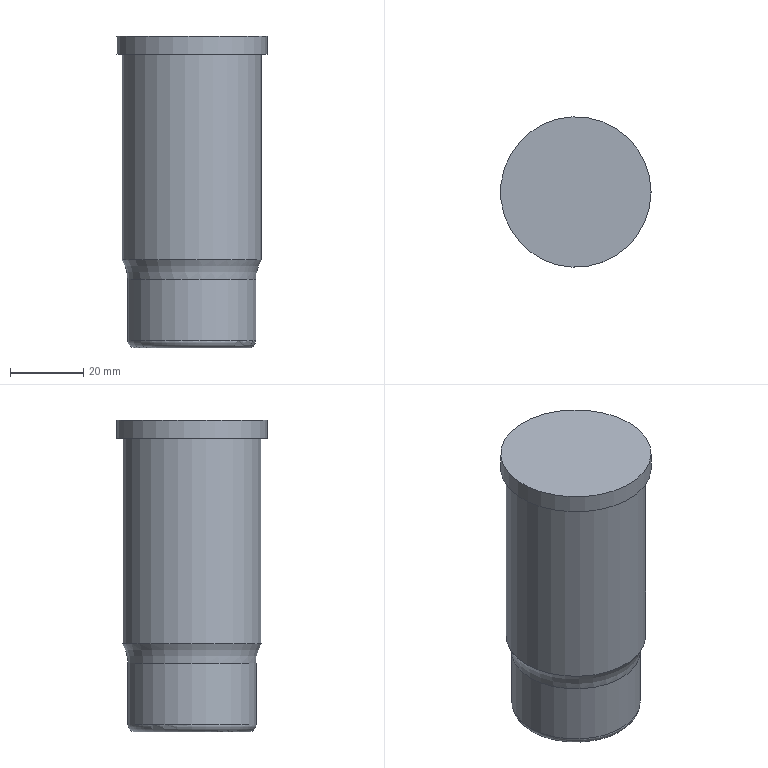Part | NX | features solid 2 | 1 solid | 8 faces | box 41 x 41 x 85 mm | volume 93398 mm3 | cylinder 3 | plane 3 | torus 2 | commonest cylinder face diameters 35 x1 38 x1 41 x1
STEP:
#1=CARTESIAN_POINT('',(1515.116,80.895,41.));
#2=VERTEX_POINT('',#1);
#3=CARTESIAN_POINT('',(1534.116,80.895,41.));
#4=DIRECTION('',(0.,0.,-1.));
#5=DIRECTION('',(-1.,0.,0.));
#6=AXIS2_PLACEMENT_3D('',#3,#4,#5);
#7=CIRCLE('',#6,19.);
#8=EDGE_CURVE('',#2,#2,#7,.T.);
#9=ORIENTED_EDGE('',*,*,#8,.F.);
#10=EDGE_LOOP('',(#9));
#11=FACE_BOUND('',#10,.T.);
#12=CARTESIAN_POINT('',(1553.116,80.895,97.));
#13=VERTEX_POINT('',#12);
#14=CARTESIAN_POINT('',(1534.116,80.895,97.));
#15=DIRECTION('',(0.,0.,-1.));
#16=DIRECTION('',(1.,0.,0.));
#17=AXIS2_PLACEMENT_3D('',#14,#15,#16);
#18=CIRCLE('',#17,19.);
#19=EDGE_CURVE('',#13,#13,#18,.T.);
#20=ORIENTED_EDGE('',*,*,#19,.T.);
#21=EDGE_LOOP('',(#20));
#22=FACE_BOUND('',#21,.T.);
#23=CARTESIAN_POINT('',(1534.116,80.895,102.));
#24=DIRECTION('',(0.,0.,-1.));
#25=DIRECTION('',(1.,0.,0.));
#26=AXIS2_PLACEMENT_3D('',#23,#24,#25);
#27=CYLINDRICAL_SURFACE('',#26,19.);
#28=ADVANCED_FACE('',(#11,#22),#27,.T.);
#29=CARTESIAN_POINT('',(1554.616,80.895,97.));
#30=VERTEX_POINT('',#29);
#31=CARTESIAN_POINT('',(1534.116,80.895,97.));
#32=DIRECTION('',(0.,0.,-1.));
#33=DIRECTION('',(1.,0.,0.));
#34=AXIS2_PLACEMENT_3D('',#31,#32,#33);
#35=CIRCLE('',#34,20.5);
#36=EDGE_CURVE('',#30,#30,#35,.T.);
#37=ORIENTED_EDGE('',*,*,#36,.T.);
#38=EDGE_LOOP('',(#37));
#39=FACE_BOUND('',#38,.T.);
#40=ORIENTED_EDGE('',*,*,#19,.F.);
#41=EDGE_LOOP('',(#40));
#42=FACE_BOUND('',#41,.T.);
#43=CARTESIAN_POINT('',(1534.116,80.895,97.));
#44=DIRECTION('',(0.,0.,1.));
#45=DIRECTION('',(-1.,0.,0.));
#46=AXIS2_PLACEMENT_3D('',#43,#44,#45);
#47=PLANE('',#46);
#48=ADVANCED_FACE('',(#39,#42),#47,.F.);
#49=ORIENTED_EDGE('',*,*,#36,.F.);
#50=EDGE_LOOP('',(#49));
#51=FACE_BOUND('',#50,.T.);
#52=CARTESIAN_POINT('',(1554.616,80.895,102.));
#53=VERTEX_POINT('',#52);
#54=CARTESIAN_POINT('',(1534.116,80.895,102.));
#55=DIRECTION('',(0.,0.,-1.));
#56=DIRECTION('',(1.,0.,0.));
#57=AXIS2_PLACEMENT_3D('',#54,#55,#56);
#58=CIRCLE('',#57,20.5);
#59=EDGE_CURVE('',#53,#53,#58,.T.);
#60=ORIENTED_EDGE('',*,*,#59,.T.);
#61=EDGE_LOOP('',(#60));
#62=FACE_BOUND('',#61,.T.);
#63=CARTESIAN_POINT('',(1534.116,80.895,99.));
#64=DIRECTION('',(0.,0.,1.));
#65=DIRECTION('',(-1.,0.,0.));
#66=AXIS2_PLACEMENT_3D('',#63,#64,#65);
#67=CYLINDRICAL_SURFACE('',#66,20.5);
#68=ADVANCED_FACE('',(#51,#62),#67,.T.);
#69=ORIENTED_EDGE('',*,*,#59,.F.);
#70=EDGE_LOOP('',(#69));
#71=FACE_BOUND('',#70,.T.);
#72=CARTESIAN_POINT('',(1534.116,80.895,102.));
#73=DIRECTION('',(0.,0.,1.));
#74=DIRECTION('',(-1.,0.,0.));
#75=AXIS2_PLACEMENT_3D('',#72,#73,#74);
#76=PLANE('',#75);
#77=ADVANCED_FACE('',(#71),#76,.T.);
#78=CARTESIAN_POINT('',(1516.616,80.895,19.));
#79=VERTEX_POINT('',#78);
#80=CARTESIAN_POINT('',(1534.116,80.895,19.));
#81=DIRECTION('',(0.,0.,-1.));
#82=DIRECTION('',(-1.,0.,0.));
#83=AXIS2_PLACEMENT_3D('',#80,#81,#82);
#84=CIRCLE('',#83,17.5);
#85=EDGE_CURVE('',#79,#79,#84,.T.);
#86=ORIENTED_EDGE('',*,*,#85,.F.);
#87=EDGE_LOOP('',(#86));
#88=FACE_BOUND('',#87,.T.);
#89=CARTESIAN_POINT('',(1516.616,80.895,35.732));
#90=VERTEX_POINT('',#89);
#91=CARTESIAN_POINT('',(1534.116,80.895,35.732));
#92=DIRECTION('',(0.,0.,-1.));
#93=DIRECTION('',(-1.,0.,0.));
#94=AXIS2_PLACEMENT_3D('',#91,#92,#93);
#95=CIRCLE('',#94,17.5);
#96=EDGE_CURVE('',#90,#90,#95,.F.);
#97=ORIENTED_EDGE('',*,*,#96,.F.);
#98=EDGE_LOOP('',(#97));
#99=FACE_BOUND('',#98,.T.);
#100=CARTESIAN_POINT('',(1534.116,80.895,22.));
#101=DIRECTION('',(0.,0.,1.));
#102=DIRECTION('',(-1.,0.,0.));
#103=AXIS2_PLACEMENT_3D('',#100,#101,#102);
#104=CYLINDRICAL_SURFACE('',#103,17.5);
#105=ADVANCED_FACE('',(#88,#99),#104,.T.);
#106=CARTESIAN_POINT('',(1518.616,80.895,17.));
#107=VERTEX_POINT('',#106);
#108=CARTESIAN_POINT('',(1534.116,80.895,17.));
#109=DIRECTION('',(0.,0.,-1.));
#110=DIRECTION('',(-1.,0.,0.));
#111=AXIS2_PLACEMENT_3D('',#108,#109,#110);
#112=CIRCLE('',#111,15.5);
#113=EDGE_CURVE('',#107,#107,#112,.F.);
#114=ORIENTED_EDGE('',*,*,#113,.F.);
#115=EDGE_LOOP('',(#114));
#116=FACE_BOUND('',#115,.T.);
#117=CARTESIAN_POINT('',(1534.116,80.895,17.));
#118=DIRECTION('',(0.,0.,1.));
#119=DIRECTION('',(-1.,0.,0.));
#120=AXIS2_PLACEMENT_3D('',#117,#118,#119);
#121=PLANE('',#120);
#122=ADVANCED_FACE('',(#116),#121,.F.);
#123=ORIENTED_EDGE('',*,*,#96,.T.);
#124=EDGE_LOOP('',(#123));
#125=FACE_BOUND('',#124,.T.);
#126=ORIENTED_EDGE('',*,*,#8,.T.);
#127=EDGE_LOOP('',(#126));
#128=FACE_BOUND('',#127,.T.);
#129=CARTESIAN_POINT('',(1534.116,80.895,35.732));
#130=DIRECTION('',(0.,0.,1.));
#131=DIRECTION('',(-1.,0.,0.));
#132=AXIS2_PLACEMENT_3D('',#129,#130,#131);
#133=TOROIDAL_SURFACE('',#132,27.5,10.);
#134=ADVANCED_FACE('',(#125,#128),#133,.F.);
#135=ORIENTED_EDGE('',*,*,#113,.T.);
#136=EDGE_LOOP('',(#135));
#137=FACE_BOUND('',#136,.T.);
#138=ORIENTED_EDGE('',*,*,#85,.T.);
#139=EDGE_LOOP('',(#138));
#140=FACE_BOUND('',#139,.T.);
#141=CARTESIAN_POINT('',(1534.116,80.895,19.));
#142=DIRECTION('',(0.,0.,1.));
#143=DIRECTION('',(-1.,0.,0.));
#144=AXIS2_PLACEMENT_3D('',#141,#142,#143);
#145=TOROIDAL_SURFACE('',#144,15.5,2.);
#146=ADVANCED_FACE('',(#137,#140),#145,.T.);
#147=CLOSED_SHELL('',(#28,#48,#68,#77,#105,#122,#134,#146));
#148=MANIFOLD_SOLID_BREP('',#147);
#149=(LENGTH_UNIT()NAMED_UNIT(*)SI_UNIT(.MILLI.,.METRE.));
#150=UNCERTAINTY_MEASURE_WITH_UNIT(LENGTH_MEASURE(0.00001),#149,'','');
#151=(NAMED_UNIT(*)PLANE_ANGLE_UNIT()SI_UNIT($,.RADIAN.));
#152=(NAMED_UNIT(*)SI_UNIT($,.STERADIAN.)SOLID_ANGLE_UNIT());
#153=(GEOMETRIC_REPRESENTATION_CONTEXT(3)GLOBAL_UNCERTAINTY_ASSIGNED_CONTEXT((#150))GLOBAL_UNIT_ASSIGNED_CONTEXT((#149,#151,#152))REPRESENTATION_CONTEXT('',''));
#154=ADVANCED_BREP_SHAPE_REPRESENTATION('',(#148),#153);